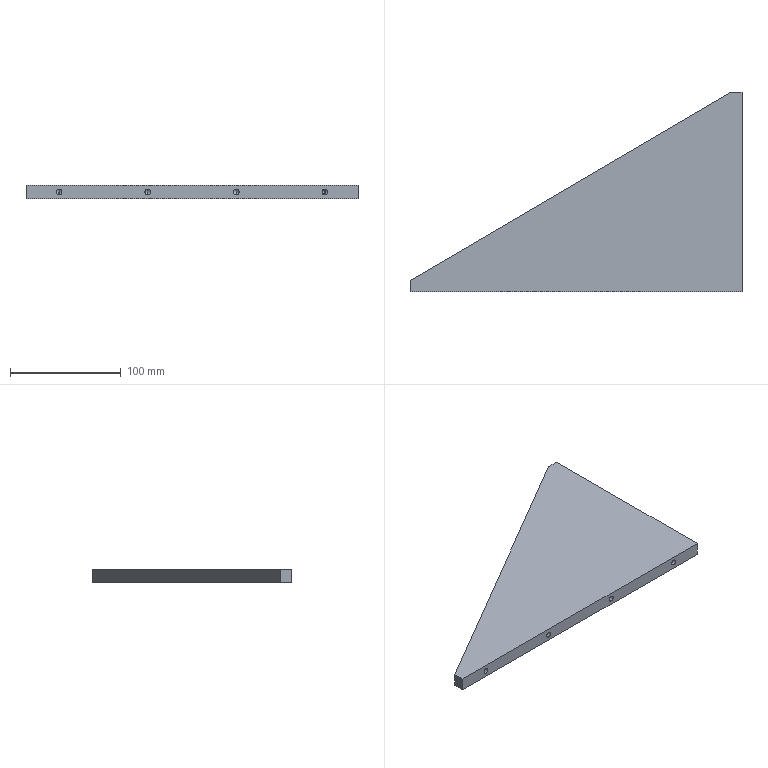Part | STEP file | KF-2212-060-003 | 1 solid | 39 faces | box 300 x 180 x 12 mm | volume 349451 mm3 | cylinder 16 | cone 16 | plane 7 | commonest cylinder face diameters 5 x16
STEP:
#1=CARTESIAN_POINT('',(270.,17.,8.5));
#2=VERTEX_POINT('',#1);
#3=CARTESIAN_POINT('',(270.,17.,3.5));
#4=VERTEX_POINT('',#3);
#5=CARTESIAN_POINT('',(270.,17.,6.));
#6=DIRECTION('',(0.,-1.,0.));
#7=DIRECTION('',(0.,0.,-1.));
#8=AXIS2_PLACEMENT_3D('',#5,#6,#7);
#9=CIRCLE('',#8,2.5);
#10=EDGE_CURVE('',#2,#4,#9,.T.);
#11=ORIENTED_EDGE('',*,*,#10,.F.);
#12=CARTESIAN_POINT('',(270.,0.,8.5));
#13=VERTEX_POINT('',#12);
#14=CARTESIAN_POINT('',(270.,0.,8.5));
#15=DIRECTION('',(0.,-1.,0.));
#16=VECTOR('',#15,1000.);
#17=LINE('',#14,#16);
#18=EDGE_CURVE('',#2,#13,#17,.T.);
#19=ORIENTED_EDGE('',*,*,#18,.T.);
#20=CARTESIAN_POINT('',(270.,0.,3.5));
#21=VERTEX_POINT('',#20);
#22=CARTESIAN_POINT('',(270.,0.,6.));
#23=DIRECTION('',(0.,-1.,0.));
#24=DIRECTION('',(0.,0.,-1.));
#25=AXIS2_PLACEMENT_3D('',#22,#23,#24);
#26=CIRCLE('',#25,2.5);
#27=EDGE_CURVE('',#13,#21,#26,.T.);
#28=ORIENTED_EDGE('',*,*,#27,.T.);
#29=CARTESIAN_POINT('',(270.,0.,3.5));
#30=DIRECTION('',(0.,-1.,0.));
#31=VECTOR('',#30,1000.);
#32=LINE('',#29,#31);
#33=EDGE_CURVE('',#4,#21,#32,.T.);
#34=ORIENTED_EDGE('',*,*,#33,.F.);
#35=EDGE_LOOP('',(#11,#19,#28,#34));
#36=FACE_OUTER_BOUND('',#35,.T.);
#37=CARTESIAN_POINT('',(270.,0.,6.));
#38=DIRECTION('',(0.,-1.,0.));
#39=DIRECTION('',(0.,0.,-1.));
#40=AXIS2_PLACEMENT_3D('',#37,#38,#39);
#41=CYLINDRICAL_SURFACE('',#40,2.5);
#42=ADVANCED_FACE('',(#36),#41,.F.);
#43=CARTESIAN_POINT('',(270.,18.502,6.));
#44=VERTEX_POINT('',#43);
#45=CARTESIAN_POINT('',(270.,17.,3.5));
#46=DIRECTION('',(0.,-0.515,-0.8572));
#47=VECTOR('',#46,1000.);
#48=LINE('',#45,#47);
#49=EDGE_CURVE('',#44,#4,#48,.T.);
#50=ORIENTED_EDGE('',*,*,#49,.F.);
#51=CARTESIAN_POINT('',(270.,17.,8.5));
#52=DIRECTION('',(0.,-0.515,0.8572));
#53=VECTOR('',#52,1000.);
#54=LINE('',#51,#53);
#55=EDGE_CURVE('',#44,#2,#54,.T.);
#56=ORIENTED_EDGE('',*,*,#55,.T.);
#57=ORIENTED_EDGE('',*,*,#10,.T.);
#58=EDGE_LOOP('',(#50,#56,#57));
#59=FACE_OUTER_BOUND('',#58,.T.);
#60=CARTESIAN_POINT('',(270.,17.,6.));
#61=DIRECTION('',(0.,-1.,0.));
#62=DIRECTION('',(0.,0.,-1.));
#63=AXIS2_PLACEMENT_3D('',#60,#61,#62);
#64=CONICAL_SURFACE('',#63,2.5,1.03);
#65=ADVANCED_FACE('',(#59),#64,.F.);
#66=CARTESIAN_POINT('',(190.,17.,8.5));
#67=VERTEX_POINT('',#66);
#68=CARTESIAN_POINT('',(190.,17.,3.5));
#69=VERTEX_POINT('',#68);
#70=CARTESIAN_POINT('',(190.,17.,6.));
#71=DIRECTION('',(0.,-1.,0.));
#72=DIRECTION('',(0.,0.,-1.));
#73=AXIS2_PLACEMENT_3D('',#70,#71,#72);
#74=CIRCLE('',#73,2.5);
#75=EDGE_CURVE('',#67,#69,#74,.T.);
#76=ORIENTED_EDGE('',*,*,#75,.F.);
#77=CARTESIAN_POINT('',(190.,0.,8.5));
#78=VERTEX_POINT('',#77);
#79=CARTESIAN_POINT('',(190.,0.,8.5));
#80=DIRECTION('',(0.,-1.,0.));
#81=VECTOR('',#80,1000.);
#82=LINE('',#79,#81);
#83=EDGE_CURVE('',#67,#78,#82,.T.);
#84=ORIENTED_EDGE('',*,*,#83,.T.);
#85=CARTESIAN_POINT('',(190.,0.,3.5));
#86=VERTEX_POINT('',#85);
#87=CARTESIAN_POINT('',(190.,0.,6.));
#88=DIRECTION('',(0.,-1.,0.));
#89=DIRECTION('',(0.,0.,-1.));
#90=AXIS2_PLACEMENT_3D('',#87,#88,#89);
#91=CIRCLE('',#90,2.5);
#92=EDGE_CURVE('',#78,#86,#91,.T.);
#93=ORIENTED_EDGE('',*,*,#92,.T.);
#94=CARTESIAN_POINT('',(190.,0.,3.5));
#95=DIRECTION('',(0.,-1.,0.));
#96=VECTOR('',#95,1000.);
#97=LINE('',#94,#96);
#98=EDGE_CURVE('',#69,#86,#97,.T.);
#99=ORIENTED_EDGE('',*,*,#98,.F.);
#100=EDGE_LOOP('',(#76,#84,#93,#99));
#101=FACE_OUTER_BOUND('',#100,.T.);
#102=CARTESIAN_POINT('',(190.,0.,6.));
#103=DIRECTION('',(0.,-1.,0.));
#104=DIRECTION('',(0.,0.,-1.));
#105=AXIS2_PLACEMENT_3D('',#102,#103,#104);
#106=CYLINDRICAL_SURFACE('',#105,2.5);
#107=ADVANCED_FACE('',(#101),#106,.F.);
#108=CARTESIAN_POINT('',(190.,18.502,6.));
#109=VERTEX_POINT('',#108);
#110=CARTESIAN_POINT('',(190.,17.,3.5));
#111=DIRECTION('',(0.,-0.515,-0.8572));
#112=VECTOR('',#111,1000.);
#113=LINE('',#110,#112);
#114=EDGE_CURVE('',#109,#69,#113,.T.);
#115=ORIENTED_EDGE('',*,*,#114,.F.);
#116=CARTESIAN_POINT('',(190.,17.,8.5));
#117=DIRECTION('',(0.,-0.515,0.8572));
#118=VECTOR('',#117,1000.);
#119=LINE('',#116,#118);
#120=EDGE_CURVE('',#109,#67,#119,.T.);
#121=ORIENTED_EDGE('',*,*,#120,.T.);
#122=ORIENTED_EDGE('',*,*,#75,.T.);
#123=EDGE_LOOP('',(#115,#121,#122));
#124=FACE_OUTER_BOUND('',#123,.T.);
#125=CARTESIAN_POINT('',(190.,17.,6.));
#126=DIRECTION('',(0.,-1.,0.));
#127=DIRECTION('',(0.,0.,-1.));
#128=AXIS2_PLACEMENT_3D('',#125,#126,#127);
#129=CONICAL_SURFACE('',#128,2.5,1.03);
#130=ADVANCED_FACE('',(#124),#129,.F.);
#131=CARTESIAN_POINT('',(110.,17.,8.5));
#132=VERTEX_POINT('',#131);
#133=CARTESIAN_POINT('',(110.,17.,3.5));
#134=VERTEX_POINT('',#133);
#135=CARTESIAN_POINT('',(110.,17.,6.));
#136=DIRECTION('',(0.,-1.,0.));
#137=DIRECTION('',(0.,0.,-1.));
#138=AXIS2_PLACEMENT_3D('',#135,#136,#137);
#139=CIRCLE('',#138,2.5);
#140=EDGE_CURVE('',#132,#134,#139,.T.);
#141=ORIENTED_EDGE('',*,*,#140,.F.);
#142=CARTESIAN_POINT('',(110.,0.,8.5));
#143=VERTEX_POINT('',#142);
#144=CARTESIAN_POINT('',(110.,0.,8.5));
#145=DIRECTION('',(0.,-1.,0.));
#146=VECTOR('',#145,1000.);
#147=LINE('',#144,#146);
#148=EDGE_CURVE('',#132,#143,#147,.T.);
#149=ORIENTED_EDGE('',*,*,#148,.T.);
#150=CARTESIAN_POINT('',(110.,0.,3.5));
#151=VERTEX_POINT('',#150);
#152=CARTESIAN_POINT('',(110.,0.,6.));
#153=DIRECTION('',(0.,-1.,0.));
#154=DIRECTION('',(0.,0.,-1.));
#155=AXIS2_PLACEMENT_3D('',#152,#153,#154);
#156=CIRCLE('',#155,2.5);
#157=EDGE_CURVE('',#143,#151,#156,.T.);
#158=ORIENTED_EDGE('',*,*,#157,.T.);
#159=CARTESIAN_POINT('',(110.,0.,3.5));
#160=DIRECTION('',(0.,-1.,0.));
#161=VECTOR('',#160,1000.);
#162=LINE('',#159,#161);
#163=EDGE_CURVE('',#134,#151,#162,.T.);
#164=ORIENTED_EDGE('',*,*,#163,.F.);
#165=EDGE_LOOP('',(#141,#149,#158,#164));
#166=FACE_OUTER_BOUND('',#165,.T.);
#167=CARTESIAN_POINT('',(110.,0.,6.));
#168=DIRECTION('',(0.,-1.,0.));
#169=DIRECTION('',(0.,0.,-1.));
#170=AXIS2_PLACEMENT_3D('',#167,#168,#169);
#171=CYLINDRICAL_SURFACE('',#170,2.5);
#172=ADVANCED_FACE('',(#166),#171,.F.);
#173=CARTESIAN_POINT('',(110.,18.502,6.));
#174=VERTEX_POINT('',#173);
#175=CARTESIAN_POINT('',(110.,17.,3.5));
#176=DIRECTION('',(0.,-0.515,-0.8572));
#177=VECTOR('',#176,1000.);
#178=LINE('',#175,#177);
#179=EDGE_CURVE('',#174,#134,#178,.T.);
#180=ORIENTED_EDGE('',*,*,#179,.F.);
#181=CARTESIAN_POINT('',(110.,17.,8.5));
#182=DIRECTION('',(0.,-0.515,0.8572));
#183=VECTOR('',#182,1000.);
#184=LINE('',#181,#183);
#185=EDGE_CURVE('',#174,#132,#184,.T.);
#186=ORIENTED_EDGE('',*,*,#185,.T.);
#187=ORIENTED_EDGE('',*,*,#140,.T.);
#188=EDGE_LOOP('',(#180,#186,#187));
#189=FACE_OUTER_BOUND('',#188,.T.);
#190=CARTESIAN_POINT('',(110.,17.,6.));
#191=DIRECTION('',(0.,-1.,0.));
#192=DIRECTION('',(0.,0.,-1.));
#193=AXIS2_PLACEMENT_3D('',#190,#191,#192);
#194=CONICAL_SURFACE('',#193,2.5,1.03);
#195=ADVANCED_FACE('',(#189),#194,.F.);
#196=CARTESIAN_POINT('',(30.,17.,8.5));
#197=VERTEX_POINT('',#196);
#198=CARTESIAN_POINT('',(30.,17.,3.5));
#199=VERTEX_POINT('',#198);
#200=CARTESIAN_POINT('',(30.,17.,6.));
#201=DIRECTION('',(0.,-1.,0.));
#202=DIRECTION('',(0.,0.,-1.));
#203=AXIS2_PLACEMENT_3D('',#200,#201,#202);
#204=CIRCLE('',#203,2.5);
#205=EDGE_CURVE('',#197,#199,#204,.T.);
#206=ORIENTED_EDGE('',*,*,#205,.F.);
#207=CARTESIAN_POINT('',(30.,0.,8.5));
#208=VERTEX_POINT('',#207);
#209=CARTESIAN_POINT('',(30.,0.,8.5));
#210=DIRECTION('',(0.,-1.,0.));
#211=VECTOR('',#210,1000.);
#212=LINE('',#209,#211);
#213=EDGE_CURVE('',#197,#208,#212,.T.);
#214=ORIENTED_EDGE('',*,*,#213,.T.);
#215=CARTESIAN_POINT('',(30.,0.,3.5));
#216=VERTEX_POINT('',#215);
#217=CARTESIAN_POINT('',(30.,0.,6.));
#218=DIRECTION('',(0.,-1.,0.));
#219=DIRECTION('',(0.,0.,-1.));
#220=AXIS2_PLACEMENT_3D('',#217,#218,#219);
#221=CIRCLE('',#220,2.5);
#222=EDGE_CURVE('',#208,#216,#221,.T.);
#223=ORIENTED_EDGE('',*,*,#222,.T.);
#224=CARTESIAN_POINT('',(30.,0.,3.5));
#225=DIRECTION('',(0.,-1.,0.));
#226=VECTOR('',#225,1000.);
#227=LINE('',#224,#226);
#228=EDGE_CURVE('',#199,#216,#227,.T.);
#229=ORIENTED_EDGE('',*,*,#228,.F.);
#230=EDGE_LOOP('',(#206,#214,#223,#229));
#231=FACE_OUTER_BOUND('',#230,.T.);
#232=CARTESIAN_POINT('',(30.,0.,6.));
#233=DIRECTION('',(0.,-1.,0.));
#234=DIRECTION('',(0.,0.,-1.));
#235=AXIS2_PLACEMENT_3D('',#232,#233,#234);
#236=CYLINDRICAL_SURFACE('',#235,2.5);
#237=ADVANCED_FACE('',(#231),#236,.F.);
#238=CARTESIAN_POINT('',(30.,18.502,6.));
#239=VERTEX_POINT('',#238);
#240=CARTESIAN_POINT('',(30.,17.,3.5));
#241=DIRECTION('',(0.,-0.515,-0.8572));
#242=VECTOR('',#241,1000.);
#243=LINE('',#240,#242);
#244=EDGE_CURVE('',#239,#199,#243,.T.);
#245=ORIENTED_EDGE('',*,*,#244,.F.);
#246=CARTESIAN_POINT('',(30.,17.,8.5));
#247=DIRECTION('',(0.,-0.515,0.8572));
#248=VECTOR('',#247,1000.);
#249=LINE('',#246,#248);
#250=EDGE_CURVE('',#239,#197,#249,.T.);
#251=ORIENTED_EDGE('',*,*,#250,.T.);
#252=ORIENTED_EDGE('',*,*,#205,.T.);
#253=EDGE_LOOP('',(#245,#251,#252));
#254=FACE_OUTER_BOUND('',#253,.T.);
#255=CARTESIAN_POINT('',(30.,17.,6.));
#256=DIRECTION('',(0.,-1.,0.));
#257=DIRECTION('',(0.,0.,-1.));
#258=AXIS2_PLACEMENT_3D('',#255,#256,#257);
#259=CONICAL_SURFACE('',#258,2.5,1.03);
#260=ADVANCED_FACE('',(#254),#259,.F.);
#261=CARTESIAN_POINT('',(283.,165.,8.5));
#262=VERTEX_POINT('',#261);
#263=CARTESIAN_POINT('',(283.,165.,3.5));
#264=VERTEX_POINT('',#263);
#265=CARTESIAN_POINT('',(283.,165.,6.));
#266=DIRECTION('',(1.,0.,0.));
#267=DIRECTION('',(0.,0.,-1.));
#268=AXIS2_PLACEMENT_3D('',#265,#266,#267);
#269=CIRCLE('',#268,2.5);
#270=EDGE_CURVE('',#262,#264,#269,.T.);
#271=ORIENTED_EDGE('',*,*,#270,.F.);
#272=CARTESIAN_POINT('',(300.,165.,8.5));
#273=VERTEX_POINT('',#272);
#274=CARTESIAN_POINT('',(300.,165.,8.5));
#275=DIRECTION('',(1.,0.,0.));
#276=VECTOR('',#275,1000.);
#277=LINE('',#274,#276);
#278=EDGE_CURVE('',#262,#273,#277,.T.);
#279=ORIENTED_EDGE('',*,*,#278,.T.);
#280=CARTESIAN_POINT('',(300.,165.,3.5));
#281=VERTEX_POINT('',#280);
#282=CARTESIAN_POINT('',(300.,165.,6.));
#283=DIRECTION('',(1.,0.,0.));
#284=DIRECTION('',(0.,0.,-1.));
#285=AXIS2_PLACEMENT_3D('',#282,#283,#284);
#286=CIRCLE('',#285,2.5);
#287=EDGE_CURVE('',#273,#281,#286,.T.);
#288=ORIENTED_EDGE('',*,*,#287,.T.);
#289=CARTESIAN_POINT('',(300.,165.,3.5));
#290=DIRECTION('',(1.,0.,0.));
#291=VECTOR('',#290,1000.);
#292=LINE('',#289,#291);
#293=EDGE_CURVE('',#264,#281,#292,.T.);
#294=ORIENTED_EDGE('',*,*,#293,.F.);
#295=EDGE_LOOP('',(#271,#279,#288,#294));
#296=FACE_OUTER_BOUND('',#295,.T.);
#297=CARTESIAN_POINT('',(300.,165.,6.));
#298=DIRECTION('',(1.,0.,0.));
#299=DIRECTION('',(0.,0.,-1.));
#300=AXIS2_PLACEMENT_3D('',#297,#298,#299);
#301=CYLINDRICAL_SURFACE('',#300,2.5);
#302=ADVANCED_FACE('',(#296),#301,.F.);
#303=CARTESIAN_POINT('',(281.498,165.,6.));
#304=VERTEX_POINT('',#303);
#305=CARTESIAN_POINT('',(283.,165.,3.5));
#306=DIRECTION('',(0.515,0.,-0.8572));
#307=VECTOR('',#306,1000.);
#308=LINE('',#305,#307);
#309=EDGE_CURVE('',#304,#264,#308,.T.);
#310=ORIENTED_EDGE('',*,*,#309,.F.);
#311=CARTESIAN_POINT('',(283.,165.,8.5));
#312=DIRECTION('',(0.515,0.,0.8572));
#313=VECTOR('',#312,1000.);
#314=LINE('',#311,#313);
#315=EDGE_CURVE('',#304,#262,#314,.T.);
#316=ORIENTED_EDGE('',*,*,#315,.T.);
#317=ORIENTED_EDGE('',*,*,#270,.T.);
#318=EDGE_LOOP('',(#310,#316,#317));
#319=FACE_OUTER_BOUND('',#318,.T.);
#320=CARTESIAN_POINT('',(283.,165.,6.));
#321=DIRECTION('',(1.,0.,0.));
#322=DIRECTION('',(0.,0.,-1.));
#323=AXIS2_PLACEMENT_3D('',#320,#321,#322);
#324=CONICAL_SURFACE('',#323,2.5,1.03);
#325=ADVANCED_FACE('',(#319),#324,.F.);
#326=CARTESIAN_POINT('',(283.,115.,8.5));
#327=VERTEX_POINT('',#326);
#328=CARTESIAN_POINT('',(283.,115.,3.5));
#329=VERTEX_POINT('',#328);
#330=CARTESIAN_POINT('',(283.,115.,6.));
#331=DIRECTION('',(1.,0.,0.));
#332=DIRECTION('',(0.,0.,-1.));
#333=AXIS2_PLACEMENT_3D('',#330,#331,#332);
#334=CIRCLE('',#333,2.5);
#335=EDGE_CURVE('',#327,#329,#334,.T.);
#336=ORIENTED_EDGE('',*,*,#335,.F.);
#337=CARTESIAN_POINT('',(300.,115.,8.5));
#338=VERTEX_POINT('',#337);
#339=CARTESIAN_POINT('',(300.,115.,8.5));
#340=DIRECTION('',(1.,0.,0.));
#341=VECTOR('',#340,1000.);
#342=LINE('',#339,#341);
#343=EDGE_CURVE('',#327,#338,#342,.T.);
#344=ORIENTED_EDGE('',*,*,#343,.T.);
#345=CARTESIAN_POINT('',(300.,115.,3.5));
#346=VERTEX_POINT('',#345);
#347=CARTESIAN_POINT('',(300.,115.,6.));
#348=DIRECTION('',(1.,0.,0.));
#349=DIRECTION('',(0.,0.,-1.));
#350=AXIS2_PLACEMENT_3D('',#347,#348,#349);
#351=CIRCLE('',#350,2.5);
#352=EDGE_CURVE('',#338,#346,#351,.T.);
#353=ORIENTED_EDGE('',*,*,#352,.T.);
#354=CARTESIAN_POINT('',(300.,115.,3.5));
#355=DIRECTION('',(1.,0.,0.));
#356=VECTOR('',#355,1000.);
#357=LINE('',#354,#356);
#358=EDGE_CURVE('',#329,#346,#357,.T.);
#359=ORIENTED_EDGE('',*,*,#358,.F.);
#360=EDGE_LOOP('',(#336,#344,#353,#359));
#361=FACE_OUTER_BOUND('',#360,.T.);
#362=CARTESIAN_POINT('',(300.,115.,6.));
#363=DIRECTION('',(1.,0.,0.));
#364=DIRECTION('',(0.,0.,-1.));
#365=AXIS2_PLACEMENT_3D('',#362,#363,#364);
#366=CYLINDRICAL_SURFACE('',#365,2.5);
#367=ADVANCED_FACE('',(#361),#366,.F.);
#368=CARTESIAN_POINT('',(281.498,115.,6.));
#369=VERTEX_POINT('',#368);
#370=CARTESIAN_POINT('',(283.,115.,3.5));
#371=DIRECTION('',(0.515,0.,-0.8572));
#372=VECTOR('',#371,1000.);
#373=LINE('',#370,#372);
#374=EDGE_CURVE('',#369,#329,#373,.T.);
#375=ORIENTED_EDGE('',*,*,#374,.F.);
#376=CARTESIAN_POINT('',(283.,115.,8.5));
#377=DIRECTION('',(0.515,0.,0.8572));
#378=VECTOR('',#377,1000.);
#379=LINE('',#376,#378);
#380=EDGE_CURVE('',#369,#327,#379,.T.);
#381=ORIENTED_EDGE('',*,*,#380,.T.);
#382=ORIENTED_EDGE('',*,*,#335,.T.);
#383=EDGE_LOOP('',(#375,#381,#382));
#384=FACE_OUTER_BOUND('',#383,.T.);
#385=CARTESIAN_POINT('',(283.,115.,6.));
#386=DIRECTION('',(1.,0.,0.));
#387=DIRECTION('',(0.,0.,-1.));
#388=AXIS2_PLACEMENT_3D('',#385,#386,#387);
#389=CONICAL_SURFACE('',#388,2.5,1.03);
#390=ADVANCED_FACE('',(#384),#389,.F.);
#391=CARTESIAN_POINT('',(283.,65.,8.5));
#392=VERTEX_POINT('',#391);
#393=CARTESIAN_POINT('',(283.,65.,3.5));
#394=VERTEX_POINT('',#393);
#395=CARTESIAN_POINT('',(283.,65.,6.));
#396=DIRECTION('',(1.,0.,0.));
#397=DIRECTION('',(0.,0.,-1.));
#398=AXIS2_PLACEMENT_3D('',#395,#396,#397);
#399=CIRCLE('',#398,2.5);
#400=EDGE_CURVE('',#392,#394,#399,.T.);
#401=ORIENTED_EDGE('',*,*,#400,.F.);
#402=CARTESIAN_POINT('',(300.,65.,8.5));
#403=VERTEX_POINT('',#402);
#404=CARTESIAN_POINT('',(300.,65.,8.5));
#405=DIRECTION('',(1.,0.,0.));
#406=VECTOR('',#405,1000.);
#407=LINE('',#404,#406);
#408=EDGE_CURVE('',#392,#403,#407,.T.);
#409=ORIENTED_EDGE('',*,*,#408,.T.);
#410=CARTESIAN_POINT('',(300.,65.,3.5));
#411=VERTEX_POINT('',#410);
#412=CARTESIAN_POINT('',(300.,65.,6.));
#413=DIRECTION('',(1.,0.,0.));
#414=DIRECTION('',(0.,0.,-1.));
#415=AXIS2_PLACEMENT_3D('',#412,#413,#414);
#416=CIRCLE('',#415,2.5);
#417=EDGE_CURVE('',#403,#411,#416,.T.);
#418=ORIENTED_EDGE('',*,*,#417,.T.);
#419=CARTESIAN_POINT('',(300.,65.,3.5));
#420=DIRECTION('',(1.,0.,0.));
#421=VECTOR('',#420,1000.);
#422=LINE('',#419,#421);
#423=EDGE_CURVE('',#394,#411,#422,.T.);
#424=ORIENTED_EDGE('',*,*,#423,.F.);
#425=EDGE_LOOP('',(#401,#409,#418,#424));
#426=FACE_OUTER_BOUND('',#425,.T.);
#427=CARTESIAN_POINT('',(300.,65.,6.));
#428=DIRECTION('',(1.,0.,0.));
#429=DIRECTION('',(0.,0.,-1.));
#430=AXIS2_PLACEMENT_3D('',#427,#428,#429);
#431=CYLINDRICAL_SURFACE('',#430,2.5);
#432=ADVANCED_FACE('',(#426),#431,.F.);
#433=CARTESIAN_POINT('',(281.498,65.,6.));
#434=VERTEX_POINT('',#433);
#435=CARTESIAN_POINT('',(283.,65.,3.5));
#436=DIRECTION('',(0.515,0.,-0.8572));
#437=VECTOR('',#436,1000.);
#438=LINE('',#435,#437);
#439=EDGE_CURVE('',#434,#394,#438,.T.);
#440=ORIENTED_EDGE('',*,*,#439,.F.);
#441=CARTESIAN_POINT('',(283.,65.,8.5));
#442=DIRECTION('',(0.515,0.,0.8572));
#443=VECTOR('',#442,1000.);
#444=LINE('',#441,#443);
#445=EDGE_CURVE('',#434,#392,#444,.T.);
#446=ORIENTED_EDGE('',*,*,#445,.T.);
#447=ORIENTED_EDGE('',*,*,#400,.T.);
#448=EDGE_LOOP('',(#440,#446,#447));
#449=FACE_OUTER_BOUND('',#448,.T.);
#450=CARTESIAN_POINT('',(283.,65.,6.));
#451=DIRECTION('',(1.,0.,0.));
#452=DIRECTION('',(0.,0.,-1.));
#453=AXIS2_PLACEMENT_3D('',#450,#451,#452);
#454=CONICAL_SURFACE('',#453,2.5,1.03);
#455=ADVANCED_FACE('',(#449),#454,.F.);
#456=CARTESIAN_POINT('',(283.,15.,8.5));
#457=VERTEX_POINT('',#456);
#458=CARTESIAN_POINT('',(283.,15.,3.5));
#459=VERTEX_POINT('',#458);
#460=CARTESIAN_POINT('',(283.,15.,6.));
#461=DIRECTION('',(1.,0.,0.));
#462=DIRECTION('',(0.,0.,-1.));
#463=AXIS2_PLACEMENT_3D('',#460,#461,#462);
#464=CIRCLE('',#463,2.5);
#465=EDGE_CURVE('',#457,#459,#464,.T.);
#466=ORIENTED_EDGE('',*,*,#465,.F.);
#467=CARTESIAN_POINT('',(300.,15.,8.5));
#468=VERTEX_POINT('',#467);
#469=CARTESIAN_POINT('',(300.,15.,8.5));
#470=DIRECTION('',(1.,0.,0.));
#471=VECTOR('',#470,1000.);
#472=LINE('',#469,#471);
#473=EDGE_CURVE('',#457,#468,#472,.T.);
#474=ORIENTED_EDGE('',*,*,#473,.T.);
#475=CARTESIAN_POINT('',(300.,15.,3.5));
#476=VERTEX_POINT('',#475);
#477=CARTESIAN_POINT('',(300.,15.,6.));
#478=DIRECTION('',(1.,0.,0.));
#479=DIRECTION('',(0.,0.,-1.));
#480=AXIS2_PLACEMENT_3D('',#477,#478,#479);
#481=CIRCLE('',#480,2.5);
#482=EDGE_CURVE('',#468,#476,#481,.T.);
#483=ORIENTED_EDGE('',*,*,#482,.T.);
#484=CARTESIAN_POINT('',(300.,15.,3.5));
#485=DIRECTION('',(1.,0.,0.));
#486=VECTOR('',#485,1000.);
#487=LINE('',#484,#486);
#488=EDGE_CURVE('',#459,#476,#487,.T.);
#489=ORIENTED_EDGE('',*,*,#488,.F.);
#490=EDGE_LOOP('',(#466,#474,#483,#489));
#491=FACE_OUTER_BOUND('',#490,.T.);
#492=CARTESIAN_POINT('',(300.,15.,6.));
#493=DIRECTION('',(1.,0.,0.));
#494=DIRECTION('',(0.,0.,-1.));
#495=AXIS2_PLACEMENT_3D('',#492,#493,#494);
#496=CYLINDRICAL_SURFACE('',#495,2.5);
#497=ADVANCED_FACE('',(#491),#496,.F.);
#498=CARTESIAN_POINT('',(281.498,15.,6.));
#499=VERTEX_POINT('',#498);
#500=CARTESIAN_POINT('',(283.,15.,3.5));
#501=DIRECTION('',(0.515,0.,-0.8572));
#502=VECTOR('',#501,1000.);
#503=LINE('',#500,#502);
#504=EDGE_CURVE('',#499,#459,#503,.T.);
#505=ORIENTED_EDGE('',*,*,#504,.F.);
#506=CARTESIAN_POINT('',(283.,15.,8.5));
#507=DIRECTION('',(0.515,0.,0.8572));
#508=VECTOR('',#507,1000.);
#509=LINE('',#506,#508);
#510=EDGE_CURVE('',#499,#457,#509,.T.);
#511=ORIENTED_EDGE('',*,*,#510,.T.);
#512=ORIENTED_EDGE('',*,*,#465,.T.);
#513=EDGE_LOOP('',(#505,#511,#512));
#514=FACE_OUTER_BOUND('',#513,.T.);
#515=CARTESIAN_POINT('',(283.,15.,6.));
#516=DIRECTION('',(1.,0.,0.));
#517=DIRECTION('',(0.,0.,-1.));
#518=AXIS2_PLACEMENT_3D('',#515,#516,#517);
#519=CONICAL_SURFACE('',#518,2.5,1.03);
#520=ADVANCED_FACE('',(#514),#519,.F.);
#521=CARTESIAN_POINT('',(190.,0.,6.));
#522=DIRECTION('',(0.,-1.,0.));
#523=DIRECTION('',(0.,0.,-1.));
#524=AXIS2_PLACEMENT_3D('',#521,#522,#523);
#525=CIRCLE('',#524,2.5);
#526=EDGE_CURVE('',#86,#78,#525,.T.);
#527=ORIENTED_EDGE('',*,*,#526,.F.);
#528=ORIENTED_EDGE('',*,*,#92,.F.);
#529=EDGE_LOOP('',(#527,#528));
#530=FACE_BOUND('',#529,.T.);
#531=CARTESIAN_POINT('',(110.,0.,6.));
#532=DIRECTION('',(0.,-1.,0.));
#533=DIRECTION('',(0.,0.,-1.));
#534=AXIS2_PLACEMENT_3D('',#531,#532,#533);
#535=CIRCLE('',#534,2.5);
#536=EDGE_CURVE('',#151,#143,#535,.T.);
#537=ORIENTED_EDGE('',*,*,#536,.F.);
#538=ORIENTED_EDGE('',*,*,#157,.F.);
#539=EDGE_LOOP('',(#537,#538));
#540=FACE_BOUND('',#539,.T.);
#541=CARTESIAN_POINT('',(30.,0.,6.));
#542=DIRECTION('',(0.,-1.,0.));
#543=DIRECTION('',(0.,0.,-1.));
#544=AXIS2_PLACEMENT_3D('',#541,#542,#543);
#545=CIRCLE('',#544,2.5);
#546=EDGE_CURVE('',#216,#208,#545,.T.);
#547=ORIENTED_EDGE('',*,*,#546,.F.);
#548=ORIENTED_EDGE('',*,*,#222,.F.);
#549=EDGE_LOOP('',(#547,#548));
#550=FACE_BOUND('',#549,.T.);
#551=CARTESIAN_POINT('',(0.,0.,0.));
#552=VERTEX_POINT('',#551);
#553=CARTESIAN_POINT('',(300.,0.,0.));
#554=VERTEX_POINT('',#553);
#555=CARTESIAN_POINT('',(0.,0.,0.));
#556=DIRECTION('',(1.,0.,0.));
#557=VECTOR('',#556,1000.);
#558=LINE('',#555,#557);
#559=EDGE_CURVE('',#552,#554,#558,.T.);
#560=ORIENTED_EDGE('',*,*,#559,.T.);
#561=CARTESIAN_POINT('',(300.,0.,12.));
#562=VERTEX_POINT('',#561);
#563=CARTESIAN_POINT('',(300.,0.,12.));
#564=DIRECTION('',(0.,0.,-1.));
#565=VECTOR('',#564,1000.);
#566=LINE('',#563,#565);
#567=EDGE_CURVE('',#562,#554,#566,.T.);
#568=ORIENTED_EDGE('',*,*,#567,.F.);
#569=CARTESIAN_POINT('',(0.,0.,12.));
#570=VERTEX_POINT('',#569);
#571=CARTESIAN_POINT('',(0.,0.,12.));
#572=DIRECTION('',(1.,0.,0.));
#573=VECTOR('',#572,1000.);
#574=LINE('',#571,#573);
#575=EDGE_CURVE('',#570,#562,#574,.T.);
#576=ORIENTED_EDGE('',*,*,#575,.F.);
#577=CARTESIAN_POINT('',(0.,0.,12.));
#578=DIRECTION('',(0.,0.,-1.));
#579=VECTOR('',#578,1000.);
#580=LINE('',#577,#579);
#581=EDGE_CURVE('',#570,#552,#580,.T.);
#582=ORIENTED_EDGE('',*,*,#581,.T.);
#583=EDGE_LOOP('',(#560,#568,#576,#582));
#584=FACE_OUTER_BOUND('',#583,.T.);
#585=CARTESIAN_POINT('',(270.,0.,6.));
#586=DIRECTION('',(0.,-1.,0.));
#587=DIRECTION('',(0.,0.,-1.));
#588=AXIS2_PLACEMENT_3D('',#585,#586,#587);
#589=CIRCLE('',#588,2.5);
#590=EDGE_CURVE('',#21,#13,#589,.T.);
#591=ORIENTED_EDGE('',*,*,#590,.F.);
#592=ORIENTED_EDGE('',*,*,#27,.F.);
#593=EDGE_LOOP('',(#591,#592));
#594=FACE_BOUND('',#593,.T.);
#595=CARTESIAN_POINT('',(0.,0.,12.));
#596=DIRECTION('',(0.,1.,0.));
#597=DIRECTION('',(0.,0.,1.));
#598=AXIS2_PLACEMENT_3D('',#595,#596,#597);
#599=PLANE('',#598);
#600=ADVANCED_FACE('',(#530,#540,#550,#584,#594),#599,.F.);
#601=CARTESIAN_POINT('',(0.,10.,0.));
#602=VERTEX_POINT('',#601);
#603=CARTESIAN_POINT('',(0.,10.,0.));
#604=DIRECTION('',(0.,-1.,0.));
#605=VECTOR('',#604,1000.);
#606=LINE('',#603,#605);
#607=EDGE_CURVE('',#602,#552,#606,.T.);
#608=ORIENTED_EDGE('',*,*,#607,.T.);
#609=ORIENTED_EDGE('',*,*,#581,.F.);
#610=CARTESIAN_POINT('',(0.,10.,12.));
#611=VERTEX_POINT('',#610);
#612=CARTESIAN_POINT('',(0.,10.,12.));
#613=DIRECTION('',(0.,-1.,0.));
#614=VECTOR('',#613,1000.);
#615=LINE('',#612,#614);
#616=EDGE_CURVE('',#611,#570,#615,.T.);
#617=ORIENTED_EDGE('',*,*,#616,.F.);
#618=CARTESIAN_POINT('',(0.,10.,12.));
#619=DIRECTION('',(0.,0.,-1.));
#620=VECTOR('',#619,1000.);
#621=LINE('',#618,#620);
#622=EDGE_CURVE('',#611,#602,#621,.T.);
#623=ORIENTED_EDGE('',*,*,#622,.T.);
#624=EDGE_LOOP('',(#608,#609,#617,#623));
#625=FACE_OUTER_BOUND('',#624,.T.);
#626=CARTESIAN_POINT('',(0.,10.,12.));
#627=DIRECTION('',(1.,0.,0.));
#628=DIRECTION('',(0.,1.,0.));
#629=AXIS2_PLACEMENT_3D('',#626,#627,#628);
#630=PLANE('',#629);
#631=ADVANCED_FACE('',(#625),#630,.F.);
#632=CARTESIAN_POINT('',(300.,165.,6.));
#633=DIRECTION('',(1.,0.,0.));
#634=DIRECTION('',(0.,0.,-1.));
#635=AXIS2_PLACEMENT_3D('',#632,#633,#634);
#636=CIRCLE('',#635,2.5);
#637=EDGE_CURVE('',#281,#273,#636,.T.);
#638=ORIENTED_EDGE('',*,*,#637,.F.);
#639=ORIENTED_EDGE('',*,*,#287,.F.);
#640=EDGE_LOOP('',(#638,#639));
#641=FACE_BOUND('',#640,.T.);
#642=CARTESIAN_POINT('',(300.,115.,6.));
#643=DIRECTION('',(1.,0.,0.));
#644=DIRECTION('',(0.,0.,-1.));
#645=AXIS2_PLACEMENT_3D('',#642,#643,#644);
#646=CIRCLE('',#645,2.5);
#647=EDGE_CURVE('',#346,#338,#646,.T.);
#648=ORIENTED_EDGE('',*,*,#647,.F.);
#649=ORIENTED_EDGE('',*,*,#352,.F.);
#650=EDGE_LOOP('',(#648,#649));
#651=FACE_BOUND('',#650,.T.);
#652=CARTESIAN_POINT('',(300.,65.,6.));
#653=DIRECTION('',(1.,0.,0.));
#654=DIRECTION('',(0.,0.,-1.));
#655=AXIS2_PLACEMENT_3D('',#652,#653,#654);
#656=CIRCLE('',#655,2.5);
#657=EDGE_CURVE('',#411,#403,#656,.T.);
#658=ORIENTED_EDGE('',*,*,#657,.F.);
#659=ORIENTED_EDGE('',*,*,#417,.F.);
#660=EDGE_LOOP('',(#658,#659));
#661=FACE_BOUND('',#660,.T.);
#662=CARTESIAN_POINT('',(300.,15.,6.));
#663=DIRECTION('',(1.,0.,0.));
#664=DIRECTION('',(0.,0.,-1.));
#665=AXIS2_PLACEMENT_3D('',#662,#663,#664);
#666=CIRCLE('',#665,2.5);
#667=EDGE_CURVE('',#476,#468,#666,.T.);
#668=ORIENTED_EDGE('',*,*,#667,.F.);
#669=ORIENTED_EDGE('',*,*,#482,.F.);
#670=EDGE_LOOP('',(#668,#669));
#671=FACE_BOUND('',#670,.T.);
#672=CARTESIAN_POINT('',(300.,180.,0.));
#673=VERTEX_POINT('',#672);
#674=CARTESIAN_POINT('',(300.,0.,0.));
#675=DIRECTION('',(0.,1.,0.));
#676=VECTOR('',#675,1000.);
#677=LINE('',#674,#676);
#678=EDGE_CURVE('',#554,#673,#677,.T.);
#679=ORIENTED_EDGE('',*,*,#678,.T.);
#680=CARTESIAN_POINT('',(300.,180.,12.));
#681=VERTEX_POINT('',#680);
#682=CARTESIAN_POINT('',(300.,180.,12.));
#683=DIRECTION('',(0.,0.,-1.));
#684=VECTOR('',#683,1000.);
#685=LINE('',#682,#684);
#686=EDGE_CURVE('',#681,#673,#685,.T.);
#687=ORIENTED_EDGE('',*,*,#686,.F.);
#688=CARTESIAN_POINT('',(300.,0.,12.));
#689=DIRECTION('',(0.,1.,0.));
#690=VECTOR('',#689,1000.);
#691=LINE('',#688,#690);
#692=EDGE_CURVE('',#562,#681,#691,.T.);
#693=ORIENTED_EDGE('',*,*,#692,.F.);
#694=ORIENTED_EDGE('',*,*,#567,.T.);
#695=EDGE_LOOP('',(#679,#687,#693,#694));
#696=FACE_OUTER_BOUND('',#695,.T.);
#697=CARTESIAN_POINT('',(300.,0.,12.));
#698=DIRECTION('',(-1.,0.,0.));
#699=DIRECTION('',(0.,0.,1.));
#700=AXIS2_PLACEMENT_3D('',#697,#698,#699);
#701=PLANE('',#700);
#702=ADVANCED_FACE('',(#641,#651,#661,#671,#696),#701,.F.);
#703=CARTESIAN_POINT('',(290.,180.,0.));
#704=VERTEX_POINT('',#703);
#705=CARTESIAN_POINT('',(300.,180.,0.));
#706=DIRECTION('',(-1.,0.,0.));
#707=VECTOR('',#706,1000.);
#708=LINE('',#705,#707);
#709=EDGE_CURVE('',#673,#704,#708,.T.);
#710=ORIENTED_EDGE('',*,*,#709,.T.);
#711=CARTESIAN_POINT('',(290.,180.,12.));
#712=VERTEX_POINT('',#711);
#713=CARTESIAN_POINT('',(290.,180.,12.));
#714=DIRECTION('',(0.,0.,-1.));
#715=VECTOR('',#714,1000.);
#716=LINE('',#713,#715);
#717=EDGE_CURVE('',#712,#704,#716,.T.);
#718=ORIENTED_EDGE('',*,*,#717,.F.);
#719=CARTESIAN_POINT('',(300.,180.,12.));
#720=DIRECTION('',(-1.,0.,0.));
#721=VECTOR('',#720,1000.);
#722=LINE('',#719,#721);
#723=EDGE_CURVE('',#681,#712,#722,.T.);
#724=ORIENTED_EDGE('',*,*,#723,.F.);
#725=ORIENTED_EDGE('',*,*,#686,.T.);
#726=EDGE_LOOP('',(#710,#718,#724,#725));
#727=FACE_OUTER_BOUND('',#726,.T.);
#728=CARTESIAN_POINT('',(300.,180.,12.));
#729=DIRECTION('',(0.,-1.,0.));
#730=DIRECTION('',(1.,0.,0.));
#731=AXIS2_PLACEMENT_3D('',#728,#729,#730);
#732=PLANE('',#731);
#733=ADVANCED_FACE('',(#727),#732,.F.);
#734=CARTESIAN_POINT('',(290.,180.,0.));
#735=DIRECTION('',(-0.8627,-0.5057,0.));
#736=VECTOR('',#735,1000.);
#737=LINE('',#734,#736);
#738=EDGE_CURVE('',#704,#602,#737,.T.);
#739=ORIENTED_EDGE('',*,*,#738,.T.);
#740=ORIENTED_EDGE('',*,*,#622,.F.);
#741=CARTESIAN_POINT('',(290.,180.,12.));
#742=DIRECTION('',(-0.8627,-0.5057,0.));
#743=VECTOR('',#742,1000.);
#744=LINE('',#741,#743);
#745=EDGE_CURVE('',#712,#611,#744,.T.);
#746=ORIENTED_EDGE('',*,*,#745,.F.);
#747=ORIENTED_EDGE('',*,*,#717,.T.);
#748=EDGE_LOOP('',(#739,#740,#746,#747));
#749=FACE_OUTER_BOUND('',#748,.T.);
#750=CARTESIAN_POINT('',(290.,180.,12.));
#751=DIRECTION('',(0.5057,-0.8627,0.));
#752=DIRECTION('',(0.8627,0.5057,0.));
#753=AXIS2_PLACEMENT_3D('',#750,#751,#752);
#754=PLANE('',#753);
#755=ADVANCED_FACE('',(#749),#754,.F.);
#756=ORIENTED_EDGE('',*,*,#616,.T.);
#757=ORIENTED_EDGE('',*,*,#575,.T.);
#758=ORIENTED_EDGE('',*,*,#692,.T.);
#759=ORIENTED_EDGE('',*,*,#723,.T.);
#760=ORIENTED_EDGE('',*,*,#745,.T.);
#761=EDGE_LOOP('',(#756,#757,#758,#759,#760));
#762=FACE_OUTER_BOUND('',#761,.T.);
#763=CARTESIAN_POINT('',(0.,0.,12.));
#764=DIRECTION('',(0.,0.,1.));
#765=DIRECTION('',(1.,0.,0.));
#766=AXIS2_PLACEMENT_3D('',#763,#764,#765);
#767=PLANE('',#766);
#768=ADVANCED_FACE('',(#762),#767,.T.);
#769=ORIENTED_EDGE('',*,*,#607,.F.);
#770=ORIENTED_EDGE('',*,*,#738,.F.);
#771=ORIENTED_EDGE('',*,*,#709,.F.);
#772=ORIENTED_EDGE('',*,*,#678,.F.);
#773=ORIENTED_EDGE('',*,*,#559,.F.);
#774=EDGE_LOOP('',(#769,#770,#771,#772,#773));
#775=FACE_OUTER_BOUND('',#774,.T.);
#776=CARTESIAN_POINT('',(0.,0.,0.));
#777=DIRECTION('',(0.,0.,1.));
#778=DIRECTION('',(1.,0.,0.));
#779=AXIS2_PLACEMENT_3D('',#776,#777,#778);
#780=PLANE('',#779);
#781=ADVANCED_FACE('',(#775),#780,.F.);
#782=ORIENTED_EDGE('',*,*,#510,.F.);
#783=ORIENTED_EDGE('',*,*,#504,.T.);
#784=CARTESIAN_POINT('',(283.,15.,6.));
#785=DIRECTION('',(1.,0.,0.));
#786=DIRECTION('',(0.,0.,-1.));
#787=AXIS2_PLACEMENT_3D('',#784,#785,#786);
#788=CIRCLE('',#787,2.5);
#789=EDGE_CURVE('',#459,#457,#788,.T.);
#790=ORIENTED_EDGE('',*,*,#789,.T.);
#791=EDGE_LOOP('',(#782,#783,#790));
#792=FACE_OUTER_BOUND('',#791,.T.);
#793=CARTESIAN_POINT('',(283.,15.,6.));
#794=DIRECTION('',(1.,0.,0.));
#795=DIRECTION('',(0.,0.,-1.));
#796=AXIS2_PLACEMENT_3D('',#793,#794,#795);
#797=CONICAL_SURFACE('',#796,2.5,1.03);
#798=ADVANCED_FACE('',(#792),#797,.F.);
#799=ORIENTED_EDGE('',*,*,#473,.F.);
#800=ORIENTED_EDGE('',*,*,#789,.F.);
#801=ORIENTED_EDGE('',*,*,#488,.T.);
#802=ORIENTED_EDGE('',*,*,#667,.T.);
#803=EDGE_LOOP('',(#799,#800,#801,#802));
#804=FACE_OUTER_BOUND('',#803,.T.);
#805=CARTESIAN_POINT('',(300.,15.,6.));
#806=DIRECTION('',(1.,0.,0.));
#807=DIRECTION('',(0.,0.,-1.));
#808=AXIS2_PLACEMENT_3D('',#805,#806,#807);
#809=CYLINDRICAL_SURFACE('',#808,2.5);
#810=ADVANCED_FACE('',(#804),#809,.F.);
#811=ORIENTED_EDGE('',*,*,#445,.F.);
#812=ORIENTED_EDGE('',*,*,#439,.T.);
#813=CARTESIAN_POINT('',(283.,65.,6.));
#814=DIRECTION('',(1.,0.,0.));
#815=DIRECTION('',(0.,0.,-1.));
#816=AXIS2_PLACEMENT_3D('',#813,#814,#815);
#817=CIRCLE('',#816,2.5);
#818=EDGE_CURVE('',#394,#392,#817,.T.);
#819=ORIENTED_EDGE('',*,*,#818,.T.);
#820=EDGE_LOOP('',(#811,#812,#819));
#821=FACE_OUTER_BOUND('',#820,.T.);
#822=CARTESIAN_POINT('',(283.,65.,6.));
#823=DIRECTION('',(1.,0.,0.));
#824=DIRECTION('',(0.,0.,-1.));
#825=AXIS2_PLACEMENT_3D('',#822,#823,#824);
#826=CONICAL_SURFACE('',#825,2.5,1.03);
#827=ADVANCED_FACE('',(#821),#826,.F.);
#828=ORIENTED_EDGE('',*,*,#408,.F.);
#829=ORIENTED_EDGE('',*,*,#818,.F.);
#830=ORIENTED_EDGE('',*,*,#423,.T.);
#831=ORIENTED_EDGE('',*,*,#657,.T.);
#832=EDGE_LOOP('',(#828,#829,#830,#831));
#833=FACE_OUTER_BOUND('',#832,.T.);
#834=CARTESIAN_POINT('',(300.,65.,6.));
#835=DIRECTION('',(1.,0.,0.));
#836=DIRECTION('',(0.,0.,-1.));
#837=AXIS2_PLACEMENT_3D('',#834,#835,#836);
#838=CYLINDRICAL_SURFACE('',#837,2.5);
#839=ADVANCED_FACE('',(#833),#838,.F.);
#840=ORIENTED_EDGE('',*,*,#380,.F.);
#841=ORIENTED_EDGE('',*,*,#374,.T.);
#842=CARTESIAN_POINT('',(283.,115.,6.));
#843=DIRECTION('',(1.,0.,0.));
#844=DIRECTION('',(0.,0.,-1.));
#845=AXIS2_PLACEMENT_3D('',#842,#843,#844);
#846=CIRCLE('',#845,2.5);
#847=EDGE_CURVE('',#329,#327,#846,.T.);
#848=ORIENTED_EDGE('',*,*,#847,.T.);
#849=EDGE_LOOP('',(#840,#841,#848));
#850=FACE_OUTER_BOUND('',#849,.T.);
#851=CARTESIAN_POINT('',(283.,115.,6.));
#852=DIRECTION('',(1.,0.,0.));
#853=DIRECTION('',(0.,0.,-1.));
#854=AXIS2_PLACEMENT_3D('',#851,#852,#853);
#855=CONICAL_SURFACE('',#854,2.5,1.03);
#856=ADVANCED_FACE('',(#850),#855,.F.);
#857=ORIENTED_EDGE('',*,*,#343,.F.);
#858=ORIENTED_EDGE('',*,*,#847,.F.);
#859=ORIENTED_EDGE('',*,*,#358,.T.);
#860=ORIENTED_EDGE('',*,*,#647,.T.);
#861=EDGE_LOOP('',(#857,#858,#859,#860));
#862=FACE_OUTER_BOUND('',#861,.T.);
#863=CARTESIAN_POINT('',(300.,115.,6.));
#864=DIRECTION('',(1.,0.,0.));
#865=DIRECTION('',(0.,0.,-1.));
#866=AXIS2_PLACEMENT_3D('',#863,#864,#865);
#867=CYLINDRICAL_SURFACE('',#866,2.5);
#868=ADVANCED_FACE('',(#862),#867,.F.);
#869=ORIENTED_EDGE('',*,*,#315,.F.);
#870=ORIENTED_EDGE('',*,*,#309,.T.);
#871=CARTESIAN_POINT('',(283.,165.,6.));
#872=DIRECTION('',(1.,0.,0.));
#873=DIRECTION('',(0.,0.,-1.));
#874=AXIS2_PLACEMENT_3D('',#871,#872,#873);
#875=CIRCLE('',#874,2.5);
#876=EDGE_CURVE('',#264,#262,#875,.T.);
#877=ORIENTED_EDGE('',*,*,#876,.T.);
#878=EDGE_LOOP('',(#869,#870,#877));
#879=FACE_OUTER_BOUND('',#878,.T.);
#880=CARTESIAN_POINT('',(283.,165.,6.));
#881=DIRECTION('',(1.,0.,0.));
#882=DIRECTION('',(0.,0.,-1.));
#883=AXIS2_PLACEMENT_3D('',#880,#881,#882);
#884=CONICAL_SURFACE('',#883,2.5,1.03);
#885=ADVANCED_FACE('',(#879),#884,.F.);
#886=ORIENTED_EDGE('',*,*,#278,.F.);
#887=ORIENTED_EDGE('',*,*,#876,.F.);
#888=ORIENTED_EDGE('',*,*,#293,.T.);
#889=ORIENTED_EDGE('',*,*,#637,.T.);
#890=EDGE_LOOP('',(#886,#887,#888,#889));
#891=FACE_OUTER_BOUND('',#890,.T.);
#892=CARTESIAN_POINT('',(300.,165.,6.));
#893=DIRECTION('',(1.,0.,0.));
#894=DIRECTION('',(0.,0.,-1.));
#895=AXIS2_PLACEMENT_3D('',#892,#893,#894);
#896=CYLINDRICAL_SURFACE('',#895,2.5);
#897=ADVANCED_FACE('',(#891),#896,.F.);
#898=ORIENTED_EDGE('',*,*,#250,.F.);
#899=ORIENTED_EDGE('',*,*,#244,.T.);
#900=CARTESIAN_POINT('',(30.,17.,6.));
#901=DIRECTION('',(0.,-1.,0.));
#902=DIRECTION('',(0.,0.,-1.));
#903=AXIS2_PLACEMENT_3D('',#900,#901,#902);
#904=CIRCLE('',#903,2.5);
#905=EDGE_CURVE('',#199,#197,#904,.T.);
#906=ORIENTED_EDGE('',*,*,#905,.T.);
#907=EDGE_LOOP('',(#898,#899,#906));
#908=FACE_OUTER_BOUND('',#907,.T.);
#909=CARTESIAN_POINT('',(30.,17.,6.));
#910=DIRECTION('',(0.,-1.,0.));
#911=DIRECTION('',(0.,0.,-1.));
#912=AXIS2_PLACEMENT_3D('',#909,#910,#911);
#913=CONICAL_SURFACE('',#912,2.5,1.03);
#914=ADVANCED_FACE('',(#908),#913,.F.);
#915=ORIENTED_EDGE('',*,*,#213,.F.);
#916=ORIENTED_EDGE('',*,*,#905,.F.);
#917=ORIENTED_EDGE('',*,*,#228,.T.);
#918=ORIENTED_EDGE('',*,*,#546,.T.);
#919=EDGE_LOOP('',(#915,#916,#917,#918));
#920=FACE_OUTER_BOUND('',#919,.T.);
#921=CARTESIAN_POINT('',(30.,0.,6.));
#922=DIRECTION('',(0.,-1.,0.));
#923=DIRECTION('',(0.,0.,-1.));
#924=AXIS2_PLACEMENT_3D('',#921,#922,#923);
#925=CYLINDRICAL_SURFACE('',#924,2.5);
#926=ADVANCED_FACE('',(#920),#925,.F.);
#927=ORIENTED_EDGE('',*,*,#185,.F.);
#928=ORIENTED_EDGE('',*,*,#179,.T.);
#929=CARTESIAN_POINT('',(110.,17.,6.));
#930=DIRECTION('',(0.,-1.,0.));
#931=DIRECTION('',(0.,0.,-1.));
#932=AXIS2_PLACEMENT_3D('',#929,#930,#931);
#933=CIRCLE('',#932,2.5);
#934=EDGE_CURVE('',#134,#132,#933,.T.);
#935=ORIENTED_EDGE('',*,*,#934,.T.);
#936=EDGE_LOOP('',(#927,#928,#935));
#937=FACE_OUTER_BOUND('',#936,.T.);
#938=CARTESIAN_POINT('',(110.,17.,6.));
#939=DIRECTION('',(0.,-1.,0.));
#940=DIRECTION('',(0.,0.,-1.));
#941=AXIS2_PLACEMENT_3D('',#938,#939,#940);
#942=CONICAL_SURFACE('',#941,2.5,1.03);
#943=ADVANCED_FACE('',(#937),#942,.F.);
#944=ORIENTED_EDGE('',*,*,#148,.F.);
#945=ORIENTED_EDGE('',*,*,#934,.F.);
#946=ORIENTED_EDGE('',*,*,#163,.T.);
#947=ORIENTED_EDGE('',*,*,#536,.T.);
#948=EDGE_LOOP('',(#944,#945,#946,#947));
#949=FACE_OUTER_BOUND('',#948,.T.);
#950=CARTESIAN_POINT('',(110.,0.,6.));
#951=DIRECTION('',(0.,-1.,0.));
#952=DIRECTION('',(0.,0.,-1.));
#953=AXIS2_PLACEMENT_3D('',#950,#951,#952);
#954=CYLINDRICAL_SURFACE('',#953,2.5);
#955=ADVANCED_FACE('',(#949),#954,.F.);
#956=ORIENTED_EDGE('',*,*,#120,.F.);
#957=ORIENTED_EDGE('',*,*,#114,.T.);
#958=CARTESIAN_POINT('',(190.,17.,6.));
#959=DIRECTION('',(0.,-1.,0.));
#960=DIRECTION('',(0.,0.,-1.));
#961=AXIS2_PLACEMENT_3D('',#958,#959,#960);
#962=CIRCLE('',#961,2.5);
#963=EDGE_CURVE('',#69,#67,#962,.T.);
#964=ORIENTED_EDGE('',*,*,#963,.T.);
#965=EDGE_LOOP('',(#956,#957,#964));
#966=FACE_OUTER_BOUND('',#965,.T.);
#967=CARTESIAN_POINT('',(190.,17.,6.));
#968=DIRECTION('',(0.,-1.,0.));
#969=DIRECTION('',(0.,0.,-1.));
#970=AXIS2_PLACEMENT_3D('',#967,#968,#969);
#971=CONICAL_SURFACE('',#970,2.5,1.03);
#972=ADVANCED_FACE('',(#966),#971,.F.);
#973=ORIENTED_EDGE('',*,*,#83,.F.);
#974=ORIENTED_EDGE('',*,*,#963,.F.);
#975=ORIENTED_EDGE('',*,*,#98,.T.);
#976=ORIENTED_EDGE('',*,*,#526,.T.);
#977=EDGE_LOOP('',(#973,#974,#975,#976));
#978=FACE_OUTER_BOUND('',#977,.T.);
#979=CARTESIAN_POINT('',(190.,0.,6.));
#980=DIRECTION('',(0.,-1.,0.));
#981=DIRECTION('',(0.,0.,-1.));
#982=AXIS2_PLACEMENT_3D('',#979,#980,#981);
#983=CYLINDRICAL_SURFACE('',#982,2.5);
#984=ADVANCED_FACE('',(#978),#983,.F.);
#985=ORIENTED_EDGE('',*,*,#55,.F.);
#986=ORIENTED_EDGE('',*,*,#49,.T.);
#987=CARTESIAN_POINT('',(270.,17.,6.));
#988=DIRECTION('',(0.,-1.,0.));
#989=DIRECTION('',(0.,0.,-1.));
#990=AXIS2_PLACEMENT_3D('',#987,#988,#989);
#991=CIRCLE('',#990,2.5);
#992=EDGE_CURVE('',#4,#2,#991,.T.);
#993=ORIENTED_EDGE('',*,*,#992,.T.);
#994=EDGE_LOOP('',(#985,#986,#993));
#995=FACE_OUTER_BOUND('',#994,.T.);
#996=CARTESIAN_POINT('',(270.,17.,6.));
#997=DIRECTION('',(0.,-1.,0.));
#998=DIRECTION('',(0.,0.,-1.));
#999=AXIS2_PLACEMENT_3D('',#996,#997,#998);
#1000=CONICAL_SURFACE('',#999,2.5,1.03);
#1001=ADVANCED_FACE('',(#995),#1000,.F.);
#1002=ORIENTED_EDGE('',*,*,#18,.F.);
#1003=ORIENTED_EDGE('',*,*,#992,.F.);
#1004=ORIENTED_EDGE('',*,*,#33,.T.);
#1005=ORIENTED_EDGE('',*,*,#590,.T.);
#1006=EDGE_LOOP('',(#1002,#1003,#1004,#1005));
#1007=FACE_OUTER_BOUND('',#1006,.T.);
#1008=CARTESIAN_POINT('',(270.,0.,6.));
#1009=DIRECTION('',(0.,-1.,0.));
#1010=DIRECTION('',(0.,0.,-1.));
#1011=AXIS2_PLACEMENT_3D('',#1008,#1009,#1010);
#1012=CYLINDRICAL_SURFACE('',#1011,2.5);
#1013=ADVANCED_FACE('',(#1007),#1012,.F.);
#1014=CLOSED_SHELL('',(#42,#65,#107,#130,#172,#195,#237,#260,#302,#325,#367,#390,#432,#455,#497,#520,#600,#631,#702,#733,#755,#768,#781,#798,#810,#827,#839,#856,#868,#885,#897,#914,#926,#943,#955,#972,#984,#1001,#1013));
#1015=MANIFOLD_SOLID_BREP('',#1014);
#1016=CARTESIAN_POINT('',(0.,0.,0.));
#1017=DIRECTION('',(0.,0.,1.));
#1018=DIRECTION('',(1.,0.,0.));
#1019=AXIS2_PLACEMENT_3D('',#1016,#1017,#1018);
#1020=(LENGTH_UNIT()NAMED_UNIT(*)SI_UNIT(.MILLI.,.METRE.));
#1021=UNCERTAINTY_MEASURE_WITH_UNIT(LENGTH_MEASURE(0.00001),#1020,'','');
#1022=(NAMED_UNIT(*)PLANE_ANGLE_UNIT()SI_UNIT($,.RADIAN.));
#1023=(NAMED_UNIT(*)SI_UNIT($,.STERADIAN.)SOLID_ANGLE_UNIT());
#1024=(GEOMETRIC_REPRESENTATION_CONTEXT(3)GLOBAL_UNCERTAINTY_ASSIGNED_CONTEXT((#1021))GLOBAL_UNIT_ASSIGNED_CONTEXT((#1020,#1022,#1023))REPRESENTATION_CONTEXT('',''));
#1025=ADVANCED_BREP_SHAPE_REPRESENTATION('',(#1015,#1019),#1024);